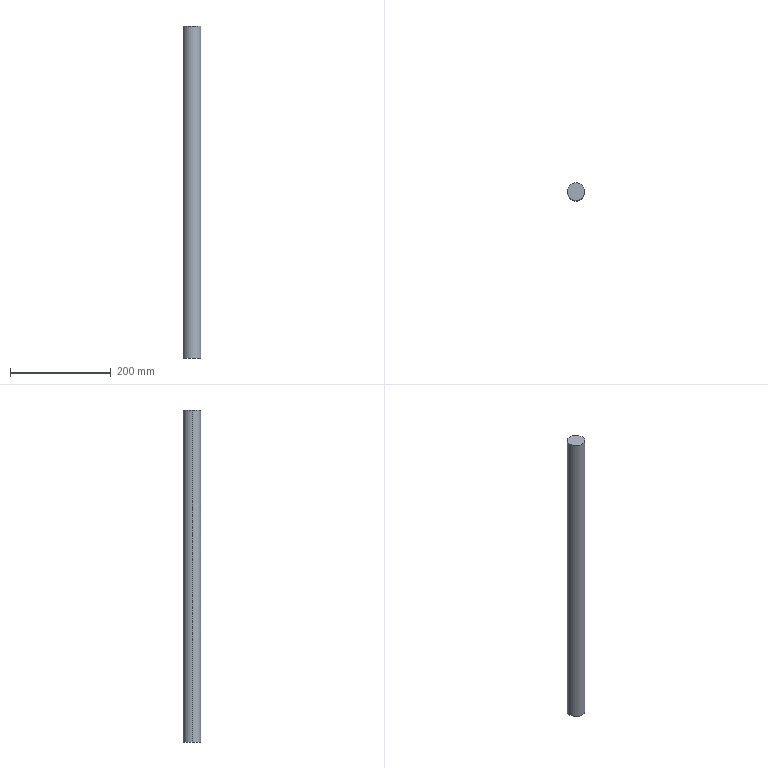Part | STEP file | Backup 2012-3-22-018 | 1 solid | 4 faces | box 35 x 35 x 658.25 mm | volume 633311 mm3 | cylinder 2 | plane 2 | commonest cylinder face diameters 35 x2
STEP:
#1=CARTESIAN_POINT('',(0.,0.,0.));
#2=DIRECTION('',(0.,0.,1.));
#3=DIRECTION('',(1.,0.,0.));
#4=AXIS2_PLACEMENT_3D('',#1,#2,#3);
#5=CARTESIAN_POINT('',(17.5,0.,658.25));
#6=VERTEX_POINT('',#5);
#7=CARTESIAN_POINT('',(-17.5,0.,658.25));
#8=VERTEX_POINT('',#7);
#9=CARTESIAN_POINT('',(0.,0.,658.25));
#10=DIRECTION('',(0.,0.,1.));
#11=DIRECTION('',(1.,0.,0.));
#12=AXIS2_PLACEMENT_3D('',#9,#10,#11);
#13=CIRCLE('',#12,17.5);
#14=CARTESIAN_POINT('',(0.,0.,658.25));
#15=DIRECTION('',(0.,0.,-1.));
#16=DIRECTION('',(-1.,0.,0.));
#17=AXIS2_PLACEMENT_3D('',#14,#15,#16);
#18=CYLINDRICAL_SURFACE('',#17,17.5);
#19=CARTESIAN_POINT('',(3.142,0.));
#20=DIRECTION('',(-1.,0.));
#21=VECTOR('',#20,1.);
#22=LINE('',#19,#21);
#23=(GEOMETRIC_REPRESENTATION_CONTEXT(2)PARAMETRIC_REPRESENTATION_CONTEXT()REPRESENTATION_CONTEXT('',''));
#24=DEFINITIONAL_REPRESENTATION('',(#22),#23);
#25=PCURVE('',#18,#24);
#26=CARTESIAN_POINT('',(0.,0.,658.25));
#27=DIRECTION('',(0.,0.,1.));
#28=DIRECTION('',(1.,0.,0.));
#29=AXIS2_PLACEMENT_3D('',#26,#27,#28);
#30=PLANE('',#29);
#31=CARTESIAN_POINT('',(0.,0.));
#32=DIRECTION('',(1.,0.));
#33=AXIS2_PLACEMENT_2D('',#31,#32);
#34=CIRCLE('',#33,17.5);
#35=(GEOMETRIC_REPRESENTATION_CONTEXT(2)PARAMETRIC_REPRESENTATION_CONTEXT()REPRESENTATION_CONTEXT('',''));
#36=DEFINITIONAL_REPRESENTATION('',(#34),#35);
#37=PCURVE('',#30,#36);
#38=SURFACE_CURVE('',#13,(#25,#37),.PCURVE_S1.);
#39=EDGE_CURVE('',#6,#8,#38,.T.);
#40=ORIENTED_EDGE('',*,*,#39,.F.);
#41=CARTESIAN_POINT('',(17.5,0.,0.));
#42=VERTEX_POINT('',#41);
#43=CARTESIAN_POINT('',(17.5,0.,658.25));
#44=DIRECTION('',(0.,0.,-1.));
#45=VECTOR('',#44,1.);
#46=LINE('',#43,#45);
#47=CARTESIAN_POINT('',(3.142,0.));
#48=DIRECTION('',(0.,1.));
#49=VECTOR('',#48,1.);
#50=LINE('',#47,#49);
#51=(GEOMETRIC_REPRESENTATION_CONTEXT(2)PARAMETRIC_REPRESENTATION_CONTEXT()REPRESENTATION_CONTEXT('',''));
#52=DEFINITIONAL_REPRESENTATION('',(#50),#51);
#53=PCURVE('',#18,#52);
#54=CARTESIAN_POINT('',(0.,0.,658.25));
#55=DIRECTION('',(0.,0.,-1.));
#56=DIRECTION('',(-1.,0.,0.));
#57=AXIS2_PLACEMENT_3D('',#54,#55,#56);
#58=CYLINDRICAL_SURFACE('',#57,17.5);
#59=CARTESIAN_POINT('',(3.142,0.));
#60=DIRECTION('',(0.,1.));
#61=VECTOR('',#60,1.);
#62=LINE('',#59,#61);
#63=(GEOMETRIC_REPRESENTATION_CONTEXT(2)PARAMETRIC_REPRESENTATION_CONTEXT()REPRESENTATION_CONTEXT('',''));
#64=DEFINITIONAL_REPRESENTATION('',(#62),#63);
#65=PCURVE('',#58,#64);
#66=SURFACE_CURVE('',#46,(#53,#65),.PCURVE_S1.);
#67=EDGE_CURVE('',#6,#42,#66,.T.);
#68=ORIENTED_EDGE('',*,*,#67,.T.);
#69=CARTESIAN_POINT('',(-17.5,0.,0.));
#70=VERTEX_POINT('',#69);
#71=CARTESIAN_POINT('',(0.,0.,0.));
#72=DIRECTION('',(0.,0.,1.));
#73=DIRECTION('',(1.,0.,0.));
#74=AXIS2_PLACEMENT_3D('',#71,#72,#73);
#75=CIRCLE('',#74,17.5);
#76=CARTESIAN_POINT('',(3.142,658.25));
#77=DIRECTION('',(-1.,0.));
#78=VECTOR('',#77,1.);
#79=LINE('',#76,#78);
#80=(GEOMETRIC_REPRESENTATION_CONTEXT(2)PARAMETRIC_REPRESENTATION_CONTEXT()REPRESENTATION_CONTEXT('',''));
#81=DEFINITIONAL_REPRESENTATION('',(#79),#80);
#82=PCURVE('',#18,#81);
#83=CARTESIAN_POINT('',(0.,0.,0.));
#84=DIRECTION('',(0.,0.,1.));
#85=DIRECTION('',(1.,0.,0.));
#86=AXIS2_PLACEMENT_3D('',#83,#84,#85);
#87=PLANE('',#86);
#88=CARTESIAN_POINT('',(0.,0.));
#89=DIRECTION('',(1.,0.));
#90=AXIS2_PLACEMENT_2D('',#88,#89);
#91=CIRCLE('',#90,17.5);
#92=(GEOMETRIC_REPRESENTATION_CONTEXT(2)PARAMETRIC_REPRESENTATION_CONTEXT()REPRESENTATION_CONTEXT('',''));
#93=DEFINITIONAL_REPRESENTATION('',(#91),#92);
#94=PCURVE('',#87,#93);
#95=SURFACE_CURVE('',#75,(#82,#94),.PCURVE_S1.);
#96=EDGE_CURVE('',#42,#70,#95,.T.);
#97=ORIENTED_EDGE('',*,*,#96,.T.);
#98=CARTESIAN_POINT('',(-17.5,0.,658.25));
#99=DIRECTION('',(0.,0.,-1.));
#100=VECTOR('',#99,1.);
#101=LINE('',#98,#100);
#102=CARTESIAN_POINT('',(0.,0.));
#103=DIRECTION('',(0.,1.));
#104=VECTOR('',#103,1.);
#105=LINE('',#102,#104);
#106=(GEOMETRIC_REPRESENTATION_CONTEXT(2)PARAMETRIC_REPRESENTATION_CONTEXT()REPRESENTATION_CONTEXT('',''));
#107=DEFINITIONAL_REPRESENTATION('',(#105),#106);
#108=PCURVE('',#18,#107);
#109=CARTESIAN_POINT('',(6.283,0.));
#110=DIRECTION('',(0.,1.));
#111=VECTOR('',#110,1.);
#112=LINE('',#109,#111);
#113=(GEOMETRIC_REPRESENTATION_CONTEXT(2)PARAMETRIC_REPRESENTATION_CONTEXT()REPRESENTATION_CONTEXT('',''));
#114=DEFINITIONAL_REPRESENTATION('',(#112),#113);
#115=PCURVE('',#58,#114);
#116=SURFACE_CURVE('',#101,(#108,#115),.PCURVE_S1.);
#117=EDGE_CURVE('',#8,#70,#116,.T.);
#118=ORIENTED_EDGE('',*,*,#117,.F.);
#119=EDGE_LOOP('',(#40,#68,#97,#118));
#120=FACE_BOUND('',#119,.T.);
#121=ADVANCED_FACE('',(#120),#18,.T.);
#122=ORIENTED_EDGE('',*,*,#67,.F.);
#123=CARTESIAN_POINT('',(0.,0.,658.25));
#124=DIRECTION('',(0.,0.,1.));
#125=DIRECTION('',(1.,0.,0.));
#126=AXIS2_PLACEMENT_3D('',#123,#124,#125);
#127=CIRCLE('',#126,17.5);
#128=CARTESIAN_POINT('',(9.425,0.));
#129=DIRECTION('',(-1.,0.));
#130=VECTOR('',#129,1.);
#131=LINE('',#128,#130);
#132=(GEOMETRIC_REPRESENTATION_CONTEXT(2)PARAMETRIC_REPRESENTATION_CONTEXT()REPRESENTATION_CONTEXT('',''));
#133=DEFINITIONAL_REPRESENTATION('',(#131),#132);
#134=PCURVE('',#58,#133);
#135=CARTESIAN_POINT('',(0.,0.));
#136=DIRECTION('',(1.,0.));
#137=AXIS2_PLACEMENT_2D('',#135,#136);
#138=CIRCLE('',#137,17.5);
#139=(GEOMETRIC_REPRESENTATION_CONTEXT(2)PARAMETRIC_REPRESENTATION_CONTEXT()REPRESENTATION_CONTEXT('',''));
#140=DEFINITIONAL_REPRESENTATION('',(#138),#139);
#141=PCURVE('',#30,#140);
#142=SURFACE_CURVE('',#127,(#134,#141),.PCURVE_S1.);
#143=EDGE_CURVE('',#8,#6,#142,.T.);
#144=ORIENTED_EDGE('',*,*,#143,.F.);
#145=ORIENTED_EDGE('',*,*,#117,.T.);
#146=CARTESIAN_POINT('',(0.,0.,0.));
#147=DIRECTION('',(0.,0.,1.));
#148=DIRECTION('',(1.,0.,0.));
#149=AXIS2_PLACEMENT_3D('',#146,#147,#148);
#150=CIRCLE('',#149,17.5);
#151=CARTESIAN_POINT('',(9.425,658.25));
#152=DIRECTION('',(-1.,0.));
#153=VECTOR('',#152,1.);
#154=LINE('',#151,#153);
#155=(GEOMETRIC_REPRESENTATION_CONTEXT(2)PARAMETRIC_REPRESENTATION_CONTEXT()REPRESENTATION_CONTEXT('',''));
#156=DEFINITIONAL_REPRESENTATION('',(#154),#155);
#157=PCURVE('',#58,#156);
#158=CARTESIAN_POINT('',(0.,0.));
#159=DIRECTION('',(1.,0.));
#160=AXIS2_PLACEMENT_2D('',#158,#159);
#161=CIRCLE('',#160,17.5);
#162=(GEOMETRIC_REPRESENTATION_CONTEXT(2)PARAMETRIC_REPRESENTATION_CONTEXT()REPRESENTATION_CONTEXT('',''));
#163=DEFINITIONAL_REPRESENTATION('',(#161),#162);
#164=PCURVE('',#87,#163);
#165=SURFACE_CURVE('',#150,(#157,#164),.PCURVE_S1.);
#166=EDGE_CURVE('',#70,#42,#165,.T.);
#167=ORIENTED_EDGE('',*,*,#166,.T.);
#168=EDGE_LOOP('',(#122,#144,#145,#167));
#169=FACE_BOUND('',#168,.T.);
#170=ADVANCED_FACE('',(#169),#58,.T.);
#171=ORIENTED_EDGE('',*,*,#143,.T.);
#172=ORIENTED_EDGE('',*,*,#39,.T.);
#173=EDGE_LOOP('',(#171,#172));
#174=FACE_BOUND('',#173,.T.);
#175=ADVANCED_FACE('',(#174),#30,.T.);
#176=ORIENTED_EDGE('',*,*,#166,.F.);
#177=ORIENTED_EDGE('',*,*,#96,.F.);
#178=EDGE_LOOP('',(#176,#177));
#179=FACE_BOUND('',#178,.T.);
#180=ADVANCED_FACE('',(#179),#87,.F.);
#181=CLOSED_SHELL('',(#121,#170,#175,#180));
#182=MANIFOLD_SOLID_BREP('',#181);
#183=(LENGTH_UNIT()NAMED_UNIT(*)SI_UNIT(.MILLI.,.METRE.));
#184=UNCERTAINTY_MEASURE_WITH_UNIT(LENGTH_MEASURE(0.0000001),#183,'','');
#185=(NAMED_UNIT(*)PLANE_ANGLE_UNIT()SI_UNIT($,.RADIAN.));
#186=(NAMED_UNIT(*)SI_UNIT($,.STERADIAN.)SOLID_ANGLE_UNIT());
#187=(GEOMETRIC_REPRESENTATION_CONTEXT(3)GLOBAL_UNCERTAINTY_ASSIGNED_CONTEXT((#184))GLOBAL_UNIT_ASSIGNED_CONTEXT((#183,#185,#186))REPRESENTATION_CONTEXT('',''));
#188=ADVANCED_BREP_SHAPE_REPRESENTATION('',(#4,#182),#187);